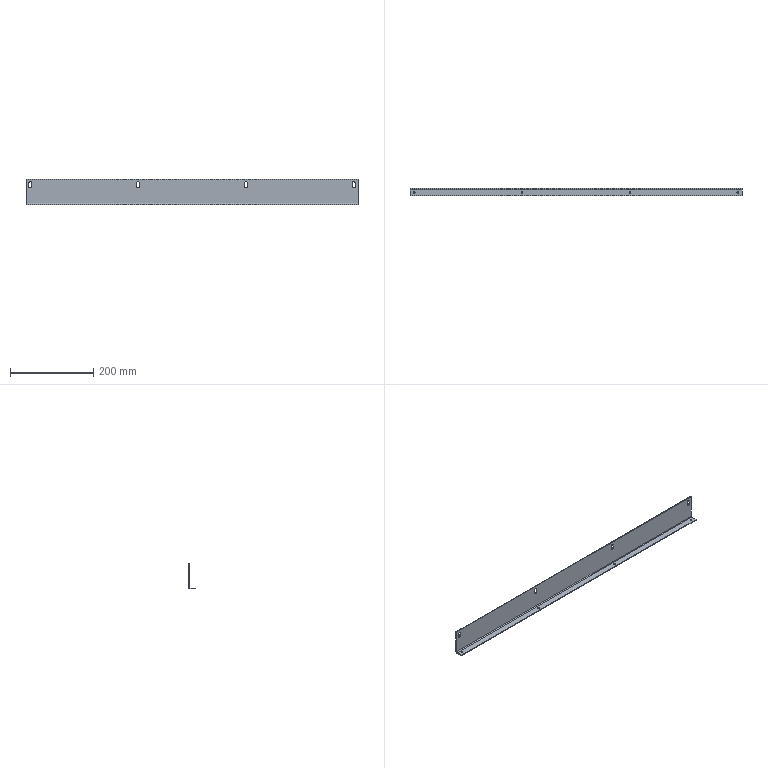Part | NX | features BREP 1 | 1 solid | 42 faces | box 800 x 18 x 62 mm | volume 121873 mm3 | cylinder 22 | plane 20 | commonest cylinder face diameters 7 x12 4.2 x8 4 x1 8 x1
STEP:
#1=CARTESIAN_POINT('',(393.5,0.,-9.5));
#2=VERTEX_POINT('',#1);
#3=CARTESIAN_POINT('',(393.5,-2.,-9.5));
#4=VERTEX_POINT('',#3);
#5=CARTESIAN_POINT('',(393.5,-18.,-9.5));
#6=DIRECTION('',(0.,-1.,0.));
#7=VECTOR('',#6,1000.);
#8=LINE('',#5,#7);
#9=EDGE_CURVE('',#2,#4,#8,.T.);
#10=ORIENTED_EDGE('',*,*,#9,.F.);
#11=CARTESIAN_POINT('',(393.5,0.,-17.5));
#12=VERTEX_POINT('',#11);
#13=CARTESIAN_POINT('',(393.5,0.,-9.5));
#14=DIRECTION('',(0.,0.,-1.));
#15=VECTOR('',#14,1000.);
#16=LINE('',#13,#15);
#17=EDGE_CURVE('',#2,#12,#16,.T.);
#18=ORIENTED_EDGE('',*,*,#17,.T.);
#19=CARTESIAN_POINT('',(393.5,-2.,-17.5));
#20=VERTEX_POINT('',#19);
#21=CARTESIAN_POINT('',(393.5,-18.,-17.5));
#22=DIRECTION('',(0.,-1.,0.));
#23=VECTOR('',#22,1000.);
#24=LINE('',#21,#23);
#25=EDGE_CURVE('',#12,#20,#24,.T.);
#26=ORIENTED_EDGE('',*,*,#25,.T.);
#27=CARTESIAN_POINT('',(393.5,-2.,0.));
#28=DIRECTION('',(0.,0.,-1.));
#29=VECTOR('',#28,1000.);
#30=LINE('',#27,#29);
#31=EDGE_CURVE('',#4,#20,#30,.T.);
#32=ORIENTED_EDGE('',*,*,#31,.F.);
#33=EDGE_LOOP('',(#10,#18,#26,#32));
#34=FACE_BOUND('',#33,.T.);
#35=CARTESIAN_POINT('',(393.5,-18.,-9.5));
#36=DIRECTION('',(1.,0.,0.));
#37=DIRECTION('',(0.,1.,0.));
#38=AXIS2_PLACEMENT_3D('',#35,#36,#37);
#39=PLANE('',#38);
#40=ADVANCED_FACE('',(#34),#39,.F.);
#41=CARTESIAN_POINT('',(386.5,-2.,-17.5));
#42=VERTEX_POINT('',#41);
#43=CARTESIAN_POINT('',(386.5,0.,-17.5));
#44=VERTEX_POINT('',#43);
#45=CARTESIAN_POINT('',(386.5,0.,-17.5));
#46=DIRECTION('',(0.,1.,0.));
#47=VECTOR('',#46,1000.);
#48=LINE('',#45,#47);
#49=EDGE_CURVE('',#42,#44,#48,.T.);
#50=ORIENTED_EDGE('',*,*,#49,.T.);
#51=CARTESIAN_POINT('',(386.5,0.,-9.5));
#52=VERTEX_POINT('',#51);
#53=CARTESIAN_POINT('',(386.5,0.,-9.5));
#54=DIRECTION('',(0.,0.,-1.));
#55=VECTOR('',#54,1000.);
#56=LINE('',#53,#55);
#57=EDGE_CURVE('',#52,#44,#56,.T.);
#58=ORIENTED_EDGE('',*,*,#57,.F.);
#59=CARTESIAN_POINT('',(386.5,-2.,-9.5));
#60=VERTEX_POINT('',#59);
#61=CARTESIAN_POINT('',(386.5,0.,-9.5));
#62=DIRECTION('',(0.,-1.,0.));
#63=VECTOR('',#62,1000.);
#64=LINE('',#61,#63);
#65=EDGE_CURVE('',#52,#60,#64,.T.);
#66=ORIENTED_EDGE('',*,*,#65,.T.);
#67=CARTESIAN_POINT('',(386.5,-2.,0.));
#68=DIRECTION('',(0.,0.,1.));
#69=VECTOR('',#68,1000.);
#70=LINE('',#67,#69);
#71=EDGE_CURVE('',#42,#60,#70,.T.);
#72=ORIENTED_EDGE('',*,*,#71,.F.);
#73=EDGE_LOOP('',(#50,#58,#66,#72));
#74=FACE_BOUND('',#73,.T.);
#75=CARTESIAN_POINT('',(386.5,0.,-9.5));
#76=DIRECTION('',(-1.,0.,0.));
#77=DIRECTION('',(0.,0.,1.));
#78=AXIS2_PLACEMENT_3D('',#75,#76,#77);
#79=PLANE('',#78);
#80=ADVANCED_FACE('',(#74),#79,.F.);
#81=CARTESIAN_POINT('',(390.,-2.,-6.));
#82=VERTEX_POINT('',#81);
#83=CARTESIAN_POINT('',(390.,0.,-6.));
#84=VERTEX_POINT('',#83);
#85=CARTESIAN_POINT('',(390.,0.,-6.));
#86=DIRECTION('',(0.,1.,0.));
#87=VECTOR('',#86,1000.);
#88=LINE('',#85,#87);
#89=EDGE_CURVE('',#82,#84,#88,.T.);
#90=ORIENTED_EDGE('',*,*,#89,.F.);
#91=CARTESIAN_POINT('',(390.,-2.,-9.5));
#92=DIRECTION('',(0.,1.,0.));
#93=DIRECTION('',(0.,0.,1.));
#94=AXIS2_PLACEMENT_3D('',#91,#92,#93);
#95=CIRCLE('',#94,3.5);
#96=EDGE_CURVE('',#60,#82,#95,.T.);
#97=ORIENTED_EDGE('',*,*,#96,.F.);
#98=ORIENTED_EDGE('',*,*,#65,.F.);
#99=CARTESIAN_POINT('',(390.,0.,-9.5));
#100=DIRECTION('',(0.,1.,0.));
#101=DIRECTION('',(0.,0.,1.));
#102=AXIS2_PLACEMENT_3D('',#99,#100,#101);
#103=CIRCLE('',#102,3.5);
#104=EDGE_CURVE('',#52,#84,#103,.T.);
#105=ORIENTED_EDGE('',*,*,#104,.T.);
#106=EDGE_LOOP('',(#90,#97,#98,#105));
#107=FACE_BOUND('',#106,.T.);
#108=CARTESIAN_POINT('',(390.,0.,-9.5));
#109=DIRECTION('',(0.,1.,0.));
#110=DIRECTION('',(0.,0.,1.));
#111=AXIS2_PLACEMENT_3D('',#108,#109,#110);
#112=CYLINDRICAL_SURFACE('',#111,3.5);
#113=ADVANCED_FACE('',(#107),#112,.F.);
#114=ORIENTED_EDGE('',*,*,#25,.F.);
#115=CARTESIAN_POINT('',(390.,0.,-17.5));
#116=DIRECTION('',(0.,1.,0.));
#117=DIRECTION('',(0.,0.,1.));
#118=AXIS2_PLACEMENT_3D('',#115,#116,#117);
#119=CIRCLE('',#118,3.5);
#120=EDGE_CURVE('',#12,#44,#119,.T.);
#121=ORIENTED_EDGE('',*,*,#120,.T.);
#122=ORIENTED_EDGE('',*,*,#49,.F.);
#123=CARTESIAN_POINT('',(390.,-2.,-17.5));
#124=DIRECTION('',(0.,1.,0.));
#125=DIRECTION('',(0.,0.,1.));
#126=AXIS2_PLACEMENT_3D('',#123,#124,#125);
#127=CIRCLE('',#126,3.5);
#128=EDGE_CURVE('',#20,#42,#127,.T.);
#129=ORIENTED_EDGE('',*,*,#128,.F.);
#130=EDGE_LOOP('',(#114,#121,#122,#129));
#131=FACE_BOUND('',#130,.T.);
#132=CARTESIAN_POINT('',(390.,0.,-17.5));
#133=DIRECTION('',(0.,1.,0.));
#134=DIRECTION('',(0.,0.,1.));
#135=AXIS2_PLACEMENT_3D('',#132,#133,#134);
#136=CYLINDRICAL_SURFACE('',#135,3.5);
#137=ADVANCED_FACE('',(#131),#136,.F.);
#138=CARTESIAN_POINT('',(133.5,0.,-9.5));
#139=VERTEX_POINT('',#138);
#140=CARTESIAN_POINT('',(133.5,-2.,-9.5));
#141=VERTEX_POINT('',#140);
#142=CARTESIAN_POINT('',(133.5,-18.,-9.5));
#143=DIRECTION('',(0.,-1.,0.));
#144=VECTOR('',#143,1000.);
#145=LINE('',#142,#144);
#146=EDGE_CURVE('',#139,#141,#145,.T.);
#147=ORIENTED_EDGE('',*,*,#146,.F.);
#148=CARTESIAN_POINT('',(133.5,0.,-17.5));
#149=VERTEX_POINT('',#148);
#150=CARTESIAN_POINT('',(133.5,0.,-9.5));
#151=DIRECTION('',(0.,0.,-1.));
#152=VECTOR('',#151,1000.);
#153=LINE('',#150,#152);
#154=EDGE_CURVE('',#139,#149,#153,.T.);
#155=ORIENTED_EDGE('',*,*,#154,.T.);
#156=CARTESIAN_POINT('',(133.5,-2.,-17.5));
#157=VERTEX_POINT('',#156);
#158=CARTESIAN_POINT('',(133.5,-18.,-17.5));
#159=DIRECTION('',(0.,-1.,0.));
#160=VECTOR('',#159,1000.);
#161=LINE('',#158,#160);
#162=EDGE_CURVE('',#149,#157,#161,.T.);
#163=ORIENTED_EDGE('',*,*,#162,.T.);
#164=CARTESIAN_POINT('',(133.5,-2.,0.));
#165=DIRECTION('',(0.,0.,-1.));
#166=VECTOR('',#165,1000.);
#167=LINE('',#164,#166);
#168=EDGE_CURVE('',#141,#157,#167,.T.);
#169=ORIENTED_EDGE('',*,*,#168,.F.);
#170=EDGE_LOOP('',(#147,#155,#163,#169));
#171=FACE_BOUND('',#170,.T.);
#172=CARTESIAN_POINT('',(133.5,-18.,-9.5));
#173=DIRECTION('',(1.,0.,0.));
#174=DIRECTION('',(0.,1.,0.));
#175=AXIS2_PLACEMENT_3D('',#172,#173,#174);
#176=PLANE('',#175);
#177=ADVANCED_FACE('',(#171),#176,.F.);
#178=CARTESIAN_POINT('',(126.5,-2.,-17.5));
#179=VERTEX_POINT('',#178);
#180=CARTESIAN_POINT('',(126.5,0.,-17.5));
#181=VERTEX_POINT('',#180);
#182=CARTESIAN_POINT('',(126.5,0.,-17.5));
#183=DIRECTION('',(0.,1.,0.));
#184=VECTOR('',#183,1000.);
#185=LINE('',#182,#184);
#186=EDGE_CURVE('',#179,#181,#185,.T.);
#187=ORIENTED_EDGE('',*,*,#186,.T.);
#188=CARTESIAN_POINT('',(126.5,0.,-9.5));
#189=VERTEX_POINT('',#188);
#190=CARTESIAN_POINT('',(126.5,0.,-9.5));
#191=DIRECTION('',(0.,0.,-1.));
#192=VECTOR('',#191,1000.);
#193=LINE('',#190,#192);
#194=EDGE_CURVE('',#189,#181,#193,.T.);
#195=ORIENTED_EDGE('',*,*,#194,.F.);
#196=CARTESIAN_POINT('',(126.5,-2.,-9.5));
#197=VERTEX_POINT('',#196);
#198=CARTESIAN_POINT('',(126.5,0.,-9.5));
#199=DIRECTION('',(0.,-1.,0.));
#200=VECTOR('',#199,1000.);
#201=LINE('',#198,#200);
#202=EDGE_CURVE('',#189,#197,#201,.T.);
#203=ORIENTED_EDGE('',*,*,#202,.T.);
#204=CARTESIAN_POINT('',(126.5,-2.,0.));
#205=DIRECTION('',(0.,0.,1.));
#206=VECTOR('',#205,1000.);
#207=LINE('',#204,#206);
#208=EDGE_CURVE('',#179,#197,#207,.T.);
#209=ORIENTED_EDGE('',*,*,#208,.F.);
#210=EDGE_LOOP('',(#187,#195,#203,#209));
#211=FACE_BOUND('',#210,.T.);
#212=CARTESIAN_POINT('',(126.5,0.,-9.5));
#213=DIRECTION('',(-1.,0.,0.));
#214=DIRECTION('',(0.,0.,1.));
#215=AXIS2_PLACEMENT_3D('',#212,#213,#214);
#216=PLANE('',#215);
#217=ADVANCED_FACE('',(#211),#216,.F.);
#218=CARTESIAN_POINT('',(130.,-2.,-6.));
#219=VERTEX_POINT('',#218);
#220=CARTESIAN_POINT('',(130.,0.,-6.));
#221=VERTEX_POINT('',#220);
#222=CARTESIAN_POINT('',(130.,0.,-6.));
#223=DIRECTION('',(0.,1.,0.));
#224=VECTOR('',#223,1000.);
#225=LINE('',#222,#224);
#226=EDGE_CURVE('',#219,#221,#225,.T.);
#227=ORIENTED_EDGE('',*,*,#226,.F.);
#228=CARTESIAN_POINT('',(130.,-2.,-9.5));
#229=DIRECTION('',(0.,1.,0.));
#230=DIRECTION('',(0.,0.,1.));
#231=AXIS2_PLACEMENT_3D('',#228,#229,#230);
#232=CIRCLE('',#231,3.5);
#233=EDGE_CURVE('',#197,#219,#232,.T.);
#234=ORIENTED_EDGE('',*,*,#233,.F.);
#235=ORIENTED_EDGE('',*,*,#202,.F.);
#236=CARTESIAN_POINT('',(130.,0.,-9.5));
#237=DIRECTION('',(0.,1.,0.));
#238=DIRECTION('',(0.,0.,1.));
#239=AXIS2_PLACEMENT_3D('',#236,#237,#238);
#240=CIRCLE('',#239,3.5);
#241=EDGE_CURVE('',#189,#221,#240,.T.);
#242=ORIENTED_EDGE('',*,*,#241,.T.);
#243=EDGE_LOOP('',(#227,#234,#235,#242));
#244=FACE_BOUND('',#243,.T.);
#245=CARTESIAN_POINT('',(130.,0.,-9.5));
#246=DIRECTION('',(0.,1.,0.));
#247=DIRECTION('',(0.,0.,1.));
#248=AXIS2_PLACEMENT_3D('',#245,#246,#247);
#249=CYLINDRICAL_SURFACE('',#248,3.5);
#250=ADVANCED_FACE('',(#244),#249,.F.);
#251=ORIENTED_EDGE('',*,*,#162,.F.);
#252=CARTESIAN_POINT('',(130.,0.,-17.5));
#253=DIRECTION('',(0.,1.,0.));
#254=DIRECTION('',(0.,0.,1.));
#255=AXIS2_PLACEMENT_3D('',#252,#253,#254);
#256=CIRCLE('',#255,3.5);
#257=EDGE_CURVE('',#149,#181,#256,.T.);
#258=ORIENTED_EDGE('',*,*,#257,.T.);
#259=ORIENTED_EDGE('',*,*,#186,.F.);
#260=CARTESIAN_POINT('',(130.,-2.,-17.5));
#261=DIRECTION('',(0.,1.,0.));
#262=DIRECTION('',(0.,0.,1.));
#263=AXIS2_PLACEMENT_3D('',#260,#261,#262);
#264=CIRCLE('',#263,3.5);
#265=EDGE_CURVE('',#157,#179,#264,.T.);
#266=ORIENTED_EDGE('',*,*,#265,.F.);
#267=EDGE_LOOP('',(#251,#258,#259,#266));
#268=FACE_BOUND('',#267,.T.);
#269=CARTESIAN_POINT('',(130.,0.,-17.5));
#270=DIRECTION('',(0.,1.,0.));
#271=DIRECTION('',(0.,0.,1.));
#272=AXIS2_PLACEMENT_3D('',#269,#270,#271);
#273=CYLINDRICAL_SURFACE('',#272,3.5);
#274=ADVANCED_FACE('',(#268),#273,.F.);
#275=CARTESIAN_POINT('',(-126.5,0.,-17.5));
#276=VERTEX_POINT('',#275);
#277=CARTESIAN_POINT('',(-126.5,-2.,-17.5));
#278=VERTEX_POINT('',#277);
#279=CARTESIAN_POINT('',(-126.5,-18.,-17.5));
#280=DIRECTION('',(0.,-1.,0.));
#281=VECTOR('',#280,1000.);
#282=LINE('',#279,#281);
#283=EDGE_CURVE('',#276,#278,#282,.T.);
#284=ORIENTED_EDGE('',*,*,#283,.F.);
#285=CARTESIAN_POINT('',(-133.5,0.,-17.5));
#286=VERTEX_POINT('',#285);
#287=CARTESIAN_POINT('',(-130.,0.,-17.5));
#288=DIRECTION('',(0.,1.,0.));
#289=DIRECTION('',(0.,0.,1.));
#290=AXIS2_PLACEMENT_3D('',#287,#288,#289);
#291=CIRCLE('',#290,3.5);
#292=EDGE_CURVE('',#276,#286,#291,.T.);
#293=ORIENTED_EDGE('',*,*,#292,.T.);
#294=CARTESIAN_POINT('',(-133.5,-2.,-17.5));
#295=VERTEX_POINT('',#294);
#296=CARTESIAN_POINT('',(-133.5,0.,-17.5));
#297=DIRECTION('',(0.,1.,0.));
#298=VECTOR('',#297,1000.);
#299=LINE('',#296,#298);
#300=EDGE_CURVE('',#295,#286,#299,.T.);
#301=ORIENTED_EDGE('',*,*,#300,.F.);
#302=CARTESIAN_POINT('',(-130.,-2.,-17.5));
#303=DIRECTION('',(0.,1.,0.));
#304=DIRECTION('',(0.,0.,1.));
#305=AXIS2_PLACEMENT_3D('',#302,#303,#304);
#306=CIRCLE('',#305,3.5);
#307=EDGE_CURVE('',#278,#295,#306,.T.);
#308=ORIENTED_EDGE('',*,*,#307,.F.);
#309=EDGE_LOOP('',(#284,#293,#301,#308));
#310=FACE_BOUND('',#309,.T.);
#311=CARTESIAN_POINT('',(-130.,0.,-17.5));
#312=DIRECTION('',(0.,1.,0.));
#313=DIRECTION('',(0.,0.,1.));
#314=AXIS2_PLACEMENT_3D('',#311,#312,#313);
#315=CYLINDRICAL_SURFACE('',#314,3.5);
#316=ADVANCED_FACE('',(#310),#315,.F.);
#317=CARTESIAN_POINT('',(-126.5,0.,-9.5));
#318=VERTEX_POINT('',#317);
#319=CARTESIAN_POINT('',(-126.5,-2.,-9.5));
#320=VERTEX_POINT('',#319);
#321=CARTESIAN_POINT('',(-126.5,-18.,-9.5));
#322=DIRECTION('',(0.,-1.,0.));
#323=VECTOR('',#322,1000.);
#324=LINE('',#321,#323);
#325=EDGE_CURVE('',#318,#320,#324,.T.);
#326=ORIENTED_EDGE('',*,*,#325,.F.);
#327=CARTESIAN_POINT('',(-126.5,0.,-9.5));
#328=DIRECTION('',(0.,0.,-1.));
#329=VECTOR('',#328,1000.);
#330=LINE('',#327,#329);
#331=EDGE_CURVE('',#318,#276,#330,.T.);
#332=ORIENTED_EDGE('',*,*,#331,.T.);
#333=ORIENTED_EDGE('',*,*,#283,.T.);
#334=CARTESIAN_POINT('',(-126.5,-2.,0.));
#335=DIRECTION('',(0.,0.,-1.));
#336=VECTOR('',#335,1000.);
#337=LINE('',#334,#336);
#338=EDGE_CURVE('',#320,#278,#337,.T.);
#339=ORIENTED_EDGE('',*,*,#338,.F.);
#340=EDGE_LOOP('',(#326,#332,#333,#339));
#341=FACE_BOUND('',#340,.T.);
#342=CARTESIAN_POINT('',(-126.5,-18.,-9.5));
#343=DIRECTION('',(1.,0.,0.));
#344=DIRECTION('',(0.,1.,0.));
#345=AXIS2_PLACEMENT_3D('',#342,#343,#344);
#346=PLANE('',#345);
#347=ADVANCED_FACE('',(#341),#346,.F.);
#348=ORIENTED_EDGE('',*,*,#300,.T.);
#349=CARTESIAN_POINT('',(-133.5,0.,-9.5));
#350=VERTEX_POINT('',#349);
#351=CARTESIAN_POINT('',(-133.5,0.,-9.5));
#352=DIRECTION('',(0.,0.,-1.));
#353=VECTOR('',#352,1000.);
#354=LINE('',#351,#353);
#355=EDGE_CURVE('',#350,#286,#354,.T.);
#356=ORIENTED_EDGE('',*,*,#355,.F.);
#357=CARTESIAN_POINT('',(-133.5,-2.,-9.5));
#358=VERTEX_POINT('',#357);
#359=CARTESIAN_POINT('',(-133.5,0.,-9.5));
#360=DIRECTION('',(0.,-1.,0.));
#361=VECTOR('',#360,1000.);
#362=LINE('',#359,#361);
#363=EDGE_CURVE('',#350,#358,#362,.T.);
#364=ORIENTED_EDGE('',*,*,#363,.T.);
#365=CARTESIAN_POINT('',(-133.5,-2.,0.));
#366=DIRECTION('',(0.,0.,1.));
#367=VECTOR('',#366,1000.);
#368=LINE('',#365,#367);
#369=EDGE_CURVE('',#295,#358,#368,.T.);
#370=ORIENTED_EDGE('',*,*,#369,.F.);
#371=EDGE_LOOP('',(#348,#356,#364,#370));
#372=FACE_BOUND('',#371,.T.);
#373=CARTESIAN_POINT('',(-133.5,0.,-9.5));
#374=DIRECTION('',(-1.,0.,0.));
#375=DIRECTION('',(0.,0.,1.));
#376=AXIS2_PLACEMENT_3D('',#373,#374,#375);
#377=PLANE('',#376);
#378=ADVANCED_FACE('',(#372),#377,.F.);
#379=CARTESIAN_POINT('',(-130.,-2.,-6.));
#380=VERTEX_POINT('',#379);
#381=CARTESIAN_POINT('',(-130.,0.,-6.));
#382=VERTEX_POINT('',#381);
#383=CARTESIAN_POINT('',(-130.,0.,-6.));
#384=DIRECTION('',(0.,1.,0.));
#385=VECTOR('',#384,1000.);
#386=LINE('',#383,#385);
#387=EDGE_CURVE('',#380,#382,#386,.T.);
#388=ORIENTED_EDGE('',*,*,#387,.F.);
#389=CARTESIAN_POINT('',(-130.,-2.,-9.5));
#390=DIRECTION('',(0.,1.,0.));
#391=DIRECTION('',(0.,0.,1.));
#392=AXIS2_PLACEMENT_3D('',#389,#390,#391);
#393=CIRCLE('',#392,3.5);
#394=EDGE_CURVE('',#358,#380,#393,.T.);
#395=ORIENTED_EDGE('',*,*,#394,.F.);
#396=ORIENTED_EDGE('',*,*,#363,.F.);
#397=CARTESIAN_POINT('',(-130.,0.,-9.5));
#398=DIRECTION('',(0.,1.,0.));
#399=DIRECTION('',(0.,0.,1.));
#400=AXIS2_PLACEMENT_3D('',#397,#398,#399);
#401=CIRCLE('',#400,3.5);
#402=EDGE_CURVE('',#350,#382,#401,.T.);
#403=ORIENTED_EDGE('',*,*,#402,.T.);
#404=EDGE_LOOP('',(#388,#395,#396,#403));
#405=FACE_BOUND('',#404,.T.);
#406=CARTESIAN_POINT('',(-130.,0.,-9.5));
#407=DIRECTION('',(0.,1.,0.));
#408=DIRECTION('',(0.,0.,1.));
#409=AXIS2_PLACEMENT_3D('',#406,#407,#408);
#410=CYLINDRICAL_SURFACE('',#409,3.5);
#411=ADVANCED_FACE('',(#405),#410,.F.);
#412=CARTESIAN_POINT('',(392.1,-10.5,-60.));
#413=VERTEX_POINT('',#412);
#414=CARTESIAN_POINT('',(392.1,-10.5,-62.));
#415=VERTEX_POINT('',#414);
#416=CARTESIAN_POINT('',(392.1,-10.5,-62.));
#417=DIRECTION('',(0.,0.,-1.));
#418=VECTOR('',#417,1000.);
#419=LINE('',#416,#418);
#420=EDGE_CURVE('',#413,#415,#419,.T.);
#421=ORIENTED_EDGE('',*,*,#420,.F.);
#422=CARTESIAN_POINT('',(387.9,-10.5,-60.));
#423=VERTEX_POINT('',#422);
#424=CARTESIAN_POINT('',(390.,-10.5,-60.));
#425=DIRECTION('',(0.,0.,-1.));
#426=DIRECTION('',(-1.,0.,0.));
#427=AXIS2_PLACEMENT_3D('',#424,#425,#426);
#428=CIRCLE('',#427,2.1);
#429=EDGE_CURVE('',#423,#413,#428,.T.);
#430=ORIENTED_EDGE('',*,*,#429,.F.);
#431=CARTESIAN_POINT('',(387.9,-10.5,-62.));
#432=VERTEX_POINT('',#431);
#433=CARTESIAN_POINT('',(387.9,-10.5,-62.));
#434=DIRECTION('',(0.,0.,-1.));
#435=VECTOR('',#434,1000.);
#436=LINE('',#433,#435);
#437=EDGE_CURVE('',#423,#432,#436,.T.);
#438=ORIENTED_EDGE('',*,*,#437,.T.);
#439=CARTESIAN_POINT('',(390.,-10.5,-62.));
#440=DIRECTION('',(0.,0.,-1.));
#441=DIRECTION('',(-1.,0.,0.));
#442=AXIS2_PLACEMENT_3D('',#439,#440,#441);
#443=CIRCLE('',#442,2.1);
#444=EDGE_CURVE('',#432,#415,#443,.T.);
#445=ORIENTED_EDGE('',*,*,#444,.T.);
#446=EDGE_LOOP('',(#421,#430,#438,#445));
#447=FACE_BOUND('',#446,.T.);
#448=CARTESIAN_POINT('',(390.,-10.5,-62.));
#449=DIRECTION('',(0.,0.,-1.));
#450=DIRECTION('',(-1.,0.,0.));
#451=AXIS2_PLACEMENT_3D('',#448,#449,#450);
#452=CYLINDRICAL_SURFACE('',#451,2.1);
#453=ADVANCED_FACE('',(#447),#452,.F.);
#454=CARTESIAN_POINT('',(132.1,-10.5,-60.));
#455=VERTEX_POINT('',#454);
#456=CARTESIAN_POINT('',(132.1,-10.5,-62.));
#457=VERTEX_POINT('',#456);
#458=CARTESIAN_POINT('',(132.1,-10.5,-62.));
#459=DIRECTION('',(0.,0.,-1.));
#460=VECTOR('',#459,1000.);
#461=LINE('',#458,#460);
#462=EDGE_CURVE('',#455,#457,#461,.T.);
#463=ORIENTED_EDGE('',*,*,#462,.F.);
#464=CARTESIAN_POINT('',(127.9,-10.5,-60.));
#465=VERTEX_POINT('',#464);
#466=CARTESIAN_POINT('',(130.,-10.5,-60.));
#467=DIRECTION('',(0.,0.,-1.));
#468=DIRECTION('',(-1.,0.,0.));
#469=AXIS2_PLACEMENT_3D('',#466,#467,#468);
#470=CIRCLE('',#469,2.1);
#471=EDGE_CURVE('',#465,#455,#470,.T.);
#472=ORIENTED_EDGE('',*,*,#471,.F.);
#473=CARTESIAN_POINT('',(127.9,-10.5,-62.));
#474=VERTEX_POINT('',#473);
#475=CARTESIAN_POINT('',(127.9,-10.5,-62.));
#476=DIRECTION('',(0.,0.,-1.));
#477=VECTOR('',#476,1000.);
#478=LINE('',#475,#477);
#479=EDGE_CURVE('',#465,#474,#478,.T.);
#480=ORIENTED_EDGE('',*,*,#479,.T.);
#481=CARTESIAN_POINT('',(130.,-10.5,-62.));
#482=DIRECTION('',(0.,0.,-1.));
#483=DIRECTION('',(-1.,0.,0.));
#484=AXIS2_PLACEMENT_3D('',#481,#482,#483);
#485=CIRCLE('',#484,2.1);
#486=EDGE_CURVE('',#474,#457,#485,.T.);
#487=ORIENTED_EDGE('',*,*,#486,.T.);
#488=EDGE_LOOP('',(#463,#472,#480,#487));
#489=FACE_BOUND('',#488,.T.);
#490=CARTESIAN_POINT('',(130.,-10.5,-62.));
#491=DIRECTION('',(0.,0.,-1.));
#492=DIRECTION('',(-1.,0.,0.));
#493=AXIS2_PLACEMENT_3D('',#490,#491,#492);
#494=CYLINDRICAL_SURFACE('',#493,2.1);
#495=ADVANCED_FACE('',(#489),#494,.F.);
#496=CARTESIAN_POINT('',(-127.9,-10.5,-60.));
#497=VERTEX_POINT('',#496);
#498=CARTESIAN_POINT('',(-127.9,-10.5,-62.));
#499=VERTEX_POINT('',#498);
#500=CARTESIAN_POINT('',(-127.9,-10.5,-62.));
#501=DIRECTION('',(0.,0.,-1.));
#502=VECTOR('',#501,1000.);
#503=LINE('',#500,#502);
#504=EDGE_CURVE('',#497,#499,#503,.T.);
#505=ORIENTED_EDGE('',*,*,#504,.F.);
#506=CARTESIAN_POINT('',(-132.1,-10.5,-60.));
#507=VERTEX_POINT('',#506);
#508=CARTESIAN_POINT('',(-130.,-10.5,-60.));
#509=DIRECTION('',(0.,0.,-1.));
#510=DIRECTION('',(-1.,0.,0.));
#511=AXIS2_PLACEMENT_3D('',#508,#509,#510);
#512=CIRCLE('',#511,2.1);
#513=EDGE_CURVE('',#507,#497,#512,.T.);
#514=ORIENTED_EDGE('',*,*,#513,.F.);
#515=CARTESIAN_POINT('',(-132.1,-10.5,-62.));
#516=VERTEX_POINT('',#515);
#517=CARTESIAN_POINT('',(-132.1,-10.5,-62.));
#518=DIRECTION('',(0.,0.,-1.));
#519=VECTOR('',#518,1000.);
#520=LINE('',#517,#519);
#521=EDGE_CURVE('',#507,#516,#520,.T.);
#522=ORIENTED_EDGE('',*,*,#521,.T.);
#523=CARTESIAN_POINT('',(-130.,-10.5,-62.));
#524=DIRECTION('',(0.,0.,-1.));
#525=DIRECTION('',(-1.,0.,0.));
#526=AXIS2_PLACEMENT_3D('',#523,#524,#525);
#527=CIRCLE('',#526,2.1);
#528=EDGE_CURVE('',#516,#499,#527,.T.);
#529=ORIENTED_EDGE('',*,*,#528,.T.);
#530=EDGE_LOOP('',(#505,#514,#522,#529));
#531=FACE_BOUND('',#530,.T.);
#532=CARTESIAN_POINT('',(-130.,-10.5,-62.));
#533=DIRECTION('',(0.,0.,-1.));
#534=DIRECTION('',(-1.,0.,0.));
#535=AXIS2_PLACEMENT_3D('',#532,#533,#534);
#536=CYLINDRICAL_SURFACE('',#535,2.1);
#537=ADVANCED_FACE('',(#531),#536,.F.);
#538=CARTESIAN_POINT('',(-393.5,-2.,-17.5));
#539=VERTEX_POINT('',#538);
#540=CARTESIAN_POINT('',(-393.5,0.,-17.5));
#541=VERTEX_POINT('',#540);
#542=CARTESIAN_POINT('',(-393.5,0.,-17.5));
#543=DIRECTION('',(0.,1.,0.));
#544=VECTOR('',#543,1000.);
#545=LINE('',#542,#544);
#546=EDGE_CURVE('',#539,#541,#545,.T.);
#547=ORIENTED_EDGE('',*,*,#546,.T.);
#548=CARTESIAN_POINT('',(-393.5,0.,-9.5));
#549=VERTEX_POINT('',#548);
#550=CARTESIAN_POINT('',(-393.5,0.,-9.5));
#551=DIRECTION('',(0.,0.,-1.));
#552=VECTOR('',#551,1000.);
#553=LINE('',#550,#552);
#554=EDGE_CURVE('',#549,#541,#553,.T.);
#555=ORIENTED_EDGE('',*,*,#554,.F.);
#556=CARTESIAN_POINT('',(-393.5,-2.,-9.5));
#557=VERTEX_POINT('',#556);
#558=CARTESIAN_POINT('',(-393.5,0.,-9.5));
#559=DIRECTION('',(0.,-1.,0.));
#560=VECTOR('',#559,1000.);
#561=LINE('',#558,#560);
#562=EDGE_CURVE('',#549,#557,#561,.T.);
#563=ORIENTED_EDGE('',*,*,#562,.T.);
#564=CARTESIAN_POINT('',(-393.5,-2.,0.));
#565=DIRECTION('',(0.,0.,1.));
#566=VECTOR('',#565,1000.);
#567=LINE('',#564,#566);
#568=EDGE_CURVE('',#539,#557,#567,.T.);
#569=ORIENTED_EDGE('',*,*,#568,.F.);
#570=EDGE_LOOP('',(#547,#555,#563,#569));
#571=FACE_BOUND('',#570,.T.);
#572=CARTESIAN_POINT('',(-393.5,0.,-9.5));
#573=DIRECTION('',(-1.,0.,0.));
#574=DIRECTION('',(0.,0.,1.));
#575=AXIS2_PLACEMENT_3D('',#572,#573,#574);
#576=PLANE('',#575);
#577=ADVANCED_FACE('',(#571),#576,.F.);
#578=CARTESIAN_POINT('',(-386.5,0.,-9.5));
#579=VERTEX_POINT('',#578);
#580=CARTESIAN_POINT('',(-386.5,-2.,-9.5));
#581=VERTEX_POINT('',#580);
#582=CARTESIAN_POINT('',(-386.5,-18.,-9.5));
#583=DIRECTION('',(0.,-1.,0.));
#584=VECTOR('',#583,1000.);
#585=LINE('',#582,#584);
#586=EDGE_CURVE('',#579,#581,#585,.T.);
#587=ORIENTED_EDGE('',*,*,#586,.F.);
#588=CARTESIAN_POINT('',(-386.5,0.,-17.5));
#589=VERTEX_POINT('',#588);
#590=CARTESIAN_POINT('',(-386.5,0.,-9.5));
#591=DIRECTION('',(0.,0.,-1.));
#592=VECTOR('',#591,1000.);
#593=LINE('',#590,#592);
#594=EDGE_CURVE('',#579,#589,#593,.T.);
#595=ORIENTED_EDGE('',*,*,#594,.T.);
#596=CARTESIAN_POINT('',(-386.5,-2.,-17.5));
#597=VERTEX_POINT('',#596);
#598=CARTESIAN_POINT('',(-386.5,-18.,-17.5));
#599=DIRECTION('',(0.,-1.,0.));
#600=VECTOR('',#599,1000.);
#601=LINE('',#598,#600);
#602=EDGE_CURVE('',#589,#597,#601,.T.);
#603=ORIENTED_EDGE('',*,*,#602,.T.);
#604=CARTESIAN_POINT('',(-386.5,-2.,0.));
#605=DIRECTION('',(0.,0.,-1.));
#606=VECTOR('',#605,1000.);
#607=LINE('',#604,#606);
#608=EDGE_CURVE('',#581,#597,#607,.T.);
#609=ORIENTED_EDGE('',*,*,#608,.F.);
#610=EDGE_LOOP('',(#587,#595,#603,#609));
#611=FACE_BOUND('',#610,.T.);
#612=CARTESIAN_POINT('',(-386.5,-18.,-9.5));
#613=DIRECTION('',(1.,0.,0.));
#614=DIRECTION('',(0.,1.,0.));
#615=AXIS2_PLACEMENT_3D('',#612,#613,#614);
#616=PLANE('',#615);
#617=ADVANCED_FACE('',(#611),#616,.F.);
#618=CARTESIAN_POINT('',(-390.,-2.,-6.));
#619=VERTEX_POINT('',#618);
#620=CARTESIAN_POINT('',(-390.,0.,-6.));
#621=VERTEX_POINT('',#620);
#622=CARTESIAN_POINT('',(-390.,0.,-6.));
#623=DIRECTION('',(0.,1.,0.));
#624=VECTOR('',#623,1000.);
#625=LINE('',#622,#624);
#626=EDGE_CURVE('',#619,#621,#625,.T.);
#627=ORIENTED_EDGE('',*,*,#626,.F.);
#628=CARTESIAN_POINT('',(-390.,-2.,-9.5));
#629=DIRECTION('',(0.,1.,0.));
#630=DIRECTION('',(0.,0.,1.));
#631=AXIS2_PLACEMENT_3D('',#628,#629,#630);
#632=CIRCLE('',#631,3.5);
#633=EDGE_CURVE('',#557,#619,#632,.T.);
#634=ORIENTED_EDGE('',*,*,#633,.F.);
#635=ORIENTED_EDGE('',*,*,#562,.F.);
#636=CARTESIAN_POINT('',(-390.,0.,-9.5));
#637=DIRECTION('',(0.,1.,0.));
#638=DIRECTION('',(0.,0.,1.));
#639=AXIS2_PLACEMENT_3D('',#636,#637,#638);
#640=CIRCLE('',#639,3.5);
#641=EDGE_CURVE('',#549,#621,#640,.T.);
#642=ORIENTED_EDGE('',*,*,#641,.T.);
#643=EDGE_LOOP('',(#627,#634,#635,#642));
#644=FACE_BOUND('',#643,.T.);
#645=CARTESIAN_POINT('',(-390.,0.,-9.5));
#646=DIRECTION('',(0.,1.,0.));
#647=DIRECTION('',(0.,0.,1.));
#648=AXIS2_PLACEMENT_3D('',#645,#646,#647);
#649=CYLINDRICAL_SURFACE('',#648,3.5);
#650=ADVANCED_FACE('',(#644),#649,.F.);
#651=ORIENTED_EDGE('',*,*,#602,.F.);
#652=CARTESIAN_POINT('',(-390.,0.,-17.5));
#653=DIRECTION('',(0.,1.,0.));
#654=DIRECTION('',(0.,0.,1.));
#655=AXIS2_PLACEMENT_3D('',#652,#653,#654);
#656=CIRCLE('',#655,3.5);
#657=EDGE_CURVE('',#589,#541,#656,.T.);
#658=ORIENTED_EDGE('',*,*,#657,.T.);
#659=ORIENTED_EDGE('',*,*,#546,.F.);
#660=CARTESIAN_POINT('',(-390.,-2.,-17.5));
#661=DIRECTION('',(0.,1.,0.));
#662=DIRECTION('',(0.,0.,1.));
#663=AXIS2_PLACEMENT_3D('',#660,#661,#662);
#664=CIRCLE('',#663,3.5);
#665=EDGE_CURVE('',#597,#539,#664,.T.);
#666=ORIENTED_EDGE('',*,*,#665,.F.);
#667=EDGE_LOOP('',(#651,#658,#659,#666));
#668=FACE_BOUND('',#667,.T.);
#669=CARTESIAN_POINT('',(-390.,0.,-17.5));
#670=DIRECTION('',(0.,1.,0.));
#671=DIRECTION('',(0.,0.,1.));
#672=AXIS2_PLACEMENT_3D('',#669,#670,#671);
#673=CYLINDRICAL_SURFACE('',#672,3.5);
#674=ADVANCED_FACE('',(#668),#673,.F.);
#675=CARTESIAN_POINT('',(-387.9,-10.5,-60.));
#676=VERTEX_POINT('',#675);
#677=CARTESIAN_POINT('',(-387.9,-10.5,-62.));
#678=VERTEX_POINT('',#677);
#679=CARTESIAN_POINT('',(-387.9,-10.5,-62.));
#680=DIRECTION('',(0.,0.,-1.));
#681=VECTOR('',#680,1000.);
#682=LINE('',#679,#681);
#683=EDGE_CURVE('',#676,#678,#682,.T.);
#684=ORIENTED_EDGE('',*,*,#683,.F.);
#685=CARTESIAN_POINT('',(-392.1,-10.5,-60.));
#686=VERTEX_POINT('',#685);
#687=CARTESIAN_POINT('',(-390.,-10.5,-60.));
#688=DIRECTION('',(0.,0.,-1.));
#689=DIRECTION('',(-1.,0.,0.));
#690=AXIS2_PLACEMENT_3D('',#687,#688,#689);
#691=CIRCLE('',#690,2.1);
#692=EDGE_CURVE('',#686,#676,#691,.T.);
#693=ORIENTED_EDGE('',*,*,#692,.F.);
#694=CARTESIAN_POINT('',(-392.1,-10.5,-62.));
#695=VERTEX_POINT('',#694);
#696=CARTESIAN_POINT('',(-392.1,-10.5,-62.));
#697=DIRECTION('',(0.,0.,-1.));
#698=VECTOR('',#697,1000.);
#699=LINE('',#696,#698);
#700=EDGE_CURVE('',#686,#695,#699,.T.);
#701=ORIENTED_EDGE('',*,*,#700,.T.);
#702=CARTESIAN_POINT('',(-390.,-10.5,-62.));
#703=DIRECTION('',(0.,0.,-1.));
#704=DIRECTION('',(-1.,0.,0.));
#705=AXIS2_PLACEMENT_3D('',#702,#703,#704);
#706=CIRCLE('',#705,2.1);
#707=EDGE_CURVE('',#695,#678,#706,.T.);
#708=ORIENTED_EDGE('',*,*,#707,.T.);
#709=EDGE_LOOP('',(#684,#693,#701,#708));
#710=FACE_BOUND('',#709,.T.);
#711=CARTESIAN_POINT('',(-390.,-10.5,-62.));
#712=DIRECTION('',(0.,0.,-1.));
#713=DIRECTION('',(-1.,0.,0.));
#714=AXIS2_PLACEMENT_3D('',#711,#712,#713);
#715=CYLINDRICAL_SURFACE('',#714,2.1);
#716=ADVANCED_FACE('',(#710),#715,.F.);
#717=CARTESIAN_POINT('',(-400.,-4.,-60.));
#718=VERTEX_POINT('',#717);
#719=CARTESIAN_POINT('',(-400.,-18.,-60.));
#720=VERTEX_POINT('',#719);
#721=CARTESIAN_POINT('',(-400.,0.,-60.));
#722=DIRECTION('',(0.,-1.,0.));
#723=VECTOR('',#722,1000.);
#724=LINE('',#721,#723);
#725=EDGE_CURVE('',#718,#720,#724,.T.);
#726=ORIENTED_EDGE('',*,*,#725,.F.);
#727=CARTESIAN_POINT('',(-400.,-4.,-62.));
#728=VERTEX_POINT('',#727);
#729=CARTESIAN_POINT('',(-400.,-4.,-60.));
#730=DIRECTION('',(0.,0.,-1.));
#731=VECTOR('',#730,1000.);
#732=LINE('',#729,#731);
#733=EDGE_CURVE('',#718,#728,#732,.T.);
#734=ORIENTED_EDGE('',*,*,#733,.T.);
#735=CARTESIAN_POINT('',(-400.,-18.,-62.));
#736=VERTEX_POINT('',#735);
#737=CARTESIAN_POINT('',(-400.,0.,-62.));
#738=DIRECTION('',(0.,-1.,0.));
#739=VECTOR('',#738,1000.);
#740=LINE('',#737,#739);
#741=EDGE_CURVE('',#728,#736,#740,.T.);
#742=ORIENTED_EDGE('',*,*,#741,.T.);
#743=CARTESIAN_POINT('',(-400.,-18.,-62.));
#744=DIRECTION('',(0.,0.,1.));
#745=VECTOR('',#744,1000.);
#746=LINE('',#743,#745);
#747=EDGE_CURVE('',#736,#720,#746,.T.);
#748=ORIENTED_EDGE('',*,*,#747,.T.);
#749=EDGE_LOOP('',(#726,#734,#742,#748));
#750=FACE_BOUND('',#749,.T.);
#751=CARTESIAN_POINT('',(-400.,-4.,-58.));
#752=DIRECTION('',(1.,0.,0.));
#753=DIRECTION('',(0.,0.,-1.));
#754=AXIS2_PLACEMENT_3D('',#751,#752,#753);
#755=PLANE('',#754);
#756=ADVANCED_FACE('',(#750),#755,.F.);
#757=CARTESIAN_POINT('',(400.,-2.,0.));
#758=VERTEX_POINT('',#757);
#759=CARTESIAN_POINT('',(400.,-2.,-58.));
#760=VERTEX_POINT('',#759);
#761=CARTESIAN_POINT('',(400.,-2.,0.));
#762=DIRECTION('',(0.,0.,-1.));
#763=VECTOR('',#762,1000.);
#764=LINE('',#761,#763);
#765=EDGE_CURVE('',#758,#760,#764,.T.);
#766=ORIENTED_EDGE('',*,*,#765,.T.);
#767=CARTESIAN_POINT('',(400.,0.,-58.));
#768=VERTEX_POINT('',#767);
#769=CARTESIAN_POINT('',(400.,-2.,-58.));
#770=DIRECTION('',(0.,1.,0.));
#771=VECTOR('',#770,1000.);
#772=LINE('',#769,#771);
#773=EDGE_CURVE('',#760,#768,#772,.T.);
#774=ORIENTED_EDGE('',*,*,#773,.T.);
#775=CARTESIAN_POINT('',(400.,0.,0.));
#776=VERTEX_POINT('',#775);
#777=CARTESIAN_POINT('',(400.,0.,0.));
#778=DIRECTION('',(0.,0.,-1.));
#779=VECTOR('',#778,1000.);
#780=LINE('',#777,#779);
#781=EDGE_CURVE('',#776,#768,#780,.T.);
#782=ORIENTED_EDGE('',*,*,#781,.F.);
#783=CARTESIAN_POINT('',(400.,-2.,0.));
#784=DIRECTION('',(0.,1.,0.));
#785=VECTOR('',#784,1000.);
#786=LINE('',#783,#785);
#787=EDGE_CURVE('',#758,#776,#786,.T.);
#788=ORIENTED_EDGE('',*,*,#787,.F.);
#789=EDGE_LOOP('',(#766,#774,#782,#788));
#790=FACE_BOUND('',#789,.T.);
#791=CARTESIAN_POINT('',(400.,-4.,-58.));
#792=DIRECTION('',(1.,0.,0.));
#793=DIRECTION('',(0.,0.,-1.));
#794=AXIS2_PLACEMENT_3D('',#791,#792,#793);
#795=PLANE('',#794);
#796=ADVANCED_FACE('',(#790),#795,.T.);
#797=CARTESIAN_POINT('',(-400.,-2.,-58.));
#798=VERTEX_POINT('',#797);
#799=CARTESIAN_POINT('',(-400.,-4.,-58.));
#800=DIRECTION('',(-1.,0.,0.));
#801=DIRECTION('',(0.,0.,-1.));
#802=AXIS2_PLACEMENT_3D('',#799,#800,#801);
#803=CIRCLE('',#802,2.);
#804=EDGE_CURVE('',#798,#718,#803,.T.);
#805=ORIENTED_EDGE('',*,*,#804,.T.);
#806=CARTESIAN_POINT('',(400.,-4.,-60.));
#807=VERTEX_POINT('',#806);
#808=CARTESIAN_POINT('',(400.,-4.,-60.));
#809=DIRECTION('',(-1.,0.,0.));
#810=VECTOR('',#809,1000.);
#811=LINE('',#808,#810);
#812=EDGE_CURVE('',#807,#718,#811,.T.);
#813=ORIENTED_EDGE('',*,*,#812,.F.);
#814=CARTESIAN_POINT('',(400.,-4.,-58.));
#815=DIRECTION('',(-1.,0.,0.));
#816=DIRECTION('',(0.,0.,-1.));
#817=AXIS2_PLACEMENT_3D('',#814,#815,#816);
#818=CIRCLE('',#817,2.);
#819=EDGE_CURVE('',#760,#807,#818,.T.);
#820=ORIENTED_EDGE('',*,*,#819,.F.);
#821=CARTESIAN_POINT('',(400.,-2.,-58.));
#822=DIRECTION('',(-1.,0.,0.));
#823=VECTOR('',#822,1000.);
#824=LINE('',#821,#823);
#825=EDGE_CURVE('',#760,#798,#824,.T.);
#826=ORIENTED_EDGE('',*,*,#825,.T.);
#827=EDGE_LOOP('',(#805,#813,#820,#826));
#828=FACE_BOUND('',#827,.T.);
#829=CARTESIAN_POINT('',(400.,-4.,-58.));
#830=DIRECTION('',(-1.,0.,0.));
#831=DIRECTION('',(0.,0.,1.));
#832=AXIS2_PLACEMENT_3D('',#829,#830,#831);
#833=CYLINDRICAL_SURFACE('',#832,2.);
#834=ADVANCED_FACE('',(#828),#833,.F.);
#835=CARTESIAN_POINT('',(-400.,-2.,0.));
#836=VERTEX_POINT('',#835);
#837=CARTESIAN_POINT('',(-400.,-2.,0.));
#838=DIRECTION('',(0.,0.,-1.));
#839=VECTOR('',#838,1000.);
#840=LINE('',#837,#839);
#841=EDGE_CURVE('',#836,#798,#840,.T.);
#842=ORIENTED_EDGE('',*,*,#841,.T.);
#843=ORIENTED_EDGE('',*,*,#825,.F.);
#844=ORIENTED_EDGE('',*,*,#765,.F.);
#845=CARTESIAN_POINT('',(400.,-2.,0.));
#846=DIRECTION('',(-1.,0.,0.));
#847=VECTOR('',#846,1000.);
#848=LINE('',#845,#847);
#849=EDGE_CURVE('',#758,#836,#848,.T.);
#850=ORIENTED_EDGE('',*,*,#849,.T.);
#851=EDGE_LOOP('',(#842,#843,#844,#850));
#852=FACE_BOUND('',#851,.T.);
#853=ORIENTED_EDGE('',*,*,#633,.T.);
#854=CARTESIAN_POINT('',(-390.,-2.,-9.5));
#855=DIRECTION('',(0.,1.,0.));
#856=DIRECTION('',(0.,0.,1.));
#857=AXIS2_PLACEMENT_3D('',#854,#855,#856);
#858=CIRCLE('',#857,3.5);
#859=EDGE_CURVE('',#619,#581,#858,.T.);
#860=ORIENTED_EDGE('',*,*,#859,.T.);
#861=ORIENTED_EDGE('',*,*,#608,.T.);
#862=ORIENTED_EDGE('',*,*,#665,.T.);
#863=ORIENTED_EDGE('',*,*,#568,.T.);
#864=EDGE_LOOP('',(#853,#860,#861,#862,#863));
#865=FACE_BOUND('',#864,.T.);
#866=ORIENTED_EDGE('',*,*,#369,.T.);
#867=ORIENTED_EDGE('',*,*,#394,.T.);
#868=CARTESIAN_POINT('',(-130.,-2.,-9.5));
#869=DIRECTION('',(0.,1.,0.));
#870=DIRECTION('',(0.,0.,1.));
#871=AXIS2_PLACEMENT_3D('',#868,#869,#870);
#872=CIRCLE('',#871,3.5);
#873=EDGE_CURVE('',#380,#320,#872,.T.);
#874=ORIENTED_EDGE('',*,*,#873,.T.);
#875=ORIENTED_EDGE('',*,*,#338,.T.);
#876=ORIENTED_EDGE('',*,*,#307,.T.);
#877=EDGE_LOOP('',(#866,#867,#874,#875,#876));
#878=FACE_BOUND('',#877,.T.);
#879=ORIENTED_EDGE('',*,*,#265,.T.);
#880=ORIENTED_EDGE('',*,*,#208,.T.);
#881=ORIENTED_EDGE('',*,*,#233,.T.);
#882=CARTESIAN_POINT('',(130.,-2.,-9.5));
#883=DIRECTION('',(0.,1.,0.));
#884=DIRECTION('',(0.,0.,1.));
#885=AXIS2_PLACEMENT_3D('',#882,#883,#884);
#886=CIRCLE('',#885,3.5);
#887=EDGE_CURVE('',#219,#141,#886,.T.);
#888=ORIENTED_EDGE('',*,*,#887,.T.);
#889=ORIENTED_EDGE('',*,*,#168,.T.);
#890=EDGE_LOOP('',(#879,#880,#881,#888,#889));
#891=FACE_BOUND('',#890,.T.);
#892=ORIENTED_EDGE('',*,*,#128,.T.);
#893=ORIENTED_EDGE('',*,*,#71,.T.);
#894=ORIENTED_EDGE('',*,*,#96,.T.);
#895=CARTESIAN_POINT('',(390.,-2.,-9.5));
#896=DIRECTION('',(0.,1.,0.));
#897=DIRECTION('',(0.,0.,1.));
#898=AXIS2_PLACEMENT_3D('',#895,#896,#897);
#899=CIRCLE('',#898,3.5);
#900=EDGE_CURVE('',#82,#4,#899,.T.);
#901=ORIENTED_EDGE('',*,*,#900,.T.);
#902=ORIENTED_EDGE('',*,*,#31,.T.);
#903=EDGE_LOOP('',(#892,#893,#894,#901,#902));
#904=FACE_BOUND('',#903,.T.);
#905=CARTESIAN_POINT('',(400.,-2.,0.));
#906=DIRECTION('',(0.,1.,0.));
#907=DIRECTION('',(0.,0.,1.));
#908=AXIS2_PLACEMENT_3D('',#905,#906,#907);
#909=PLANE('',#908);
#910=ADVANCED_FACE('',(#852,#865,#878,#891,#904),#909,.F.);
#911=CARTESIAN_POINT('',(-400.,0.,0.));
#912=VERTEX_POINT('',#911);
#913=CARTESIAN_POINT('',(-400.,-2.,0.));
#914=DIRECTION('',(0.,1.,0.));
#915=VECTOR('',#914,1000.);
#916=LINE('',#913,#915);
#917=EDGE_CURVE('',#836,#912,#916,.T.);
#918=ORIENTED_EDGE('',*,*,#917,.F.);
#919=ORIENTED_EDGE('',*,*,#849,.F.);
#920=ORIENTED_EDGE('',*,*,#787,.T.);
#921=CARTESIAN_POINT('',(400.,0.,0.));
#922=DIRECTION('',(-1.,0.,0.));
#923=VECTOR('',#922,1000.);
#924=LINE('',#921,#923);
#925=EDGE_CURVE('',#776,#912,#924,.T.);
#926=ORIENTED_EDGE('',*,*,#925,.T.);
#927=EDGE_LOOP('',(#918,#919,#920,#926));
#928=FACE_BOUND('',#927,.T.);
#929=CARTESIAN_POINT('',(400.,-2.,0.));
#930=DIRECTION('',(0.,0.,1.));
#931=DIRECTION('',(1.,0.,0.));
#932=AXIS2_PLACEMENT_3D('',#929,#930,#931);
#933=PLANE('',#932);
#934=ADVANCED_FACE('',(#928),#933,.T.);
#935=CARTESIAN_POINT('',(-400.,0.,-58.));
#936=VERTEX_POINT('',#935);
#937=CARTESIAN_POINT('',(-400.,-4.,-58.));
#938=DIRECTION('',(-1.,0.,0.));
#939=DIRECTION('',(0.,0.,-1.));
#940=AXIS2_PLACEMENT_3D('',#937,#938,#939);
#941=CIRCLE('',#940,4.);
#942=EDGE_CURVE('',#936,#728,#941,.T.);
#943=ORIENTED_EDGE('',*,*,#942,.F.);
#944=CARTESIAN_POINT('',(400.,0.,-58.));
#945=DIRECTION('',(-1.,0.,0.));
#946=VECTOR('',#945,1000.);
#947=LINE('',#944,#946);
#948=EDGE_CURVE('',#768,#936,#947,.T.);
#949=ORIENTED_EDGE('',*,*,#948,.F.);
#950=CARTESIAN_POINT('',(400.,-4.,-62.));
#951=VERTEX_POINT('',#950);
#952=CARTESIAN_POINT('',(400.,-4.,-58.));
#953=DIRECTION('',(-1.,0.,0.));
#954=DIRECTION('',(0.,0.,-1.));
#955=AXIS2_PLACEMENT_3D('',#952,#953,#954);
#956=CIRCLE('',#955,4.);
#957=EDGE_CURVE('',#768,#951,#956,.T.);
#958=ORIENTED_EDGE('',*,*,#957,.T.);
#959=CARTESIAN_POINT('',(400.,-4.,-62.));
#960=DIRECTION('',(-1.,0.,0.));
#961=VECTOR('',#960,1000.);
#962=LINE('',#959,#961);
#963=EDGE_CURVE('',#951,#728,#962,.T.);
#964=ORIENTED_EDGE('',*,*,#963,.T.);
#965=EDGE_LOOP('',(#943,#949,#958,#964));
#966=FACE_BOUND('',#965,.T.);
#967=CARTESIAN_POINT('',(400.,-4.,-58.));
#968=DIRECTION('',(-1.,0.,0.));
#969=DIRECTION('',(0.,0.,1.));
#970=AXIS2_PLACEMENT_3D('',#967,#968,#969);
#971=CYLINDRICAL_SURFACE('',#970,4.);
#972=ADVANCED_FACE('',(#966),#971,.T.);
#973=ORIENTED_EDGE('',*,*,#741,.F.);
#974=ORIENTED_EDGE('',*,*,#963,.F.);
#975=CARTESIAN_POINT('',(400.,-18.,-62.));
#976=VERTEX_POINT('',#975);
#977=CARTESIAN_POINT('',(400.,0.,-62.));
#978=DIRECTION('',(0.,-1.,0.));
#979=VECTOR('',#978,1000.);
#980=LINE('',#977,#979);
#981=EDGE_CURVE('',#951,#976,#980,.T.);
#982=ORIENTED_EDGE('',*,*,#981,.T.);
#983=CARTESIAN_POINT('',(400.,-18.,-62.));
#984=DIRECTION('',(-1.,0.,0.));
#985=VECTOR('',#984,1000.);
#986=LINE('',#983,#985);
#987=EDGE_CURVE('',#976,#736,#986,.T.);
#988=ORIENTED_EDGE('',*,*,#987,.T.);
#989=EDGE_LOOP('',(#973,#974,#982,#988));
#990=FACE_BOUND('',#989,.T.);
#991=ORIENTED_EDGE('',*,*,#707,.F.);
#992=CARTESIAN_POINT('',(-390.,-10.5,-62.));
#993=DIRECTION('',(0.,0.,-1.));
#994=DIRECTION('',(-1.,0.,0.));
#995=AXIS2_PLACEMENT_3D('',#992,#993,#994);
#996=CIRCLE('',#995,2.1);
#997=EDGE_CURVE('',#678,#695,#996,.T.);
#998=ORIENTED_EDGE('',*,*,#997,.F.);
#999=EDGE_LOOP('',(#991,#998));
#1000=FACE_BOUND('',#999,.T.);
#1001=ORIENTED_EDGE('',*,*,#528,.F.);
#1002=CARTESIAN_POINT('',(-130.,-10.5,-62.));
#1003=DIRECTION('',(0.,0.,-1.));
#1004=DIRECTION('',(-1.,0.,0.));
#1005=AXIS2_PLACEMENT_3D('',#1002,#1003,#1004);
#1006=CIRCLE('',#1005,2.1);
#1007=EDGE_CURVE('',#499,#516,#1006,.T.);
#1008=ORIENTED_EDGE('',*,*,#1007,.F.);
#1009=EDGE_LOOP('',(#1001,#1008));
#1010=FACE_BOUND('',#1009,.T.);
#1011=ORIENTED_EDGE('',*,*,#486,.F.);
#1012=CARTESIAN_POINT('',(130.,-10.5,-62.));
#1013=DIRECTION('',(0.,0.,-1.));
#1014=DIRECTION('',(-1.,0.,0.));
#1015=AXIS2_PLACEMENT_3D('',#1012,#1013,#1014);
#1016=CIRCLE('',#1015,2.1);
#1017=EDGE_CURVE('',#457,#474,#1016,.T.);
#1018=ORIENTED_EDGE('',*,*,#1017,.F.);
#1019=EDGE_LOOP('',(#1011,#1018));
#1020=FACE_BOUND('',#1019,.T.);
#1021=ORIENTED_EDGE('',*,*,#444,.F.);
#1022=CARTESIAN_POINT('',(390.,-10.5,-62.));
#1023=DIRECTION('',(0.,0.,-1.));
#1024=DIRECTION('',(-1.,0.,0.));
#1025=AXIS2_PLACEMENT_3D('',#1022,#1023,#1024);
#1026=CIRCLE('',#1025,2.1);
#1027=EDGE_CURVE('',#415,#432,#1026,.T.);
#1028=ORIENTED_EDGE('',*,*,#1027,.F.);
#1029=EDGE_LOOP('',(#1021,#1028));
#1030=FACE_BOUND('',#1029,.T.);
#1031=CARTESIAN_POINT('',(400.,0.,-62.));
#1032=DIRECTION('',(0.,0.,-1.));
#1033=DIRECTION('',(-1.,0.,0.));
#1034=AXIS2_PLACEMENT_3D('',#1031,#1032,#1033);
#1035=PLANE('',#1034);
#1036=ADVANCED_FACE('',(#990,#1000,#1010,#1020,#1030),#1035,.T.);
#1037=ORIENTED_EDGE('',*,*,#747,.F.);
#1038=ORIENTED_EDGE('',*,*,#987,.F.);
#1039=CARTESIAN_POINT('',(400.,-18.,-60.));
#1040=VERTEX_POINT('',#1039);
#1041=CARTESIAN_POINT('',(400.,-18.,-62.));
#1042=DIRECTION('',(0.,0.,1.));
#1043=VECTOR('',#1042,1000.);
#1044=LINE('',#1041,#1043);
#1045=EDGE_CURVE('',#976,#1040,#1044,.T.);
#1046=ORIENTED_EDGE('',*,*,#1045,.T.);
#1047=CARTESIAN_POINT('',(400.,-18.,-60.));
#1048=DIRECTION('',(-1.,0.,0.));
#1049=VECTOR('',#1048,1000.);
#1050=LINE('',#1047,#1049);
#1051=EDGE_CURVE('',#1040,#720,#1050,.T.);
#1052=ORIENTED_EDGE('',*,*,#1051,.T.);
#1053=EDGE_LOOP('',(#1037,#1038,#1046,#1052));
#1054=FACE_BOUND('',#1053,.T.);
#1055=CARTESIAN_POINT('',(400.,-18.,-62.));
#1056=DIRECTION('',(0.,-1.,0.));
#1057=DIRECTION('',(0.,0.,-1.));
#1058=AXIS2_PLACEMENT_3D('',#1055,#1056,#1057);
#1059=PLANE('',#1058);
#1060=ADVANCED_FACE('',(#1054),#1059,.T.);
#1061=ORIENTED_EDGE('',*,*,#725,.T.);
#1062=ORIENTED_EDGE('',*,*,#1051,.F.);
#1063=CARTESIAN_POINT('',(400.,0.,-60.));
#1064=DIRECTION('',(0.,-1.,0.));
#1065=VECTOR('',#1064,1000.);
#1066=LINE('',#1063,#1065);
#1067=EDGE_CURVE('',#807,#1040,#1066,.T.);
#1068=ORIENTED_EDGE('',*,*,#1067,.F.);
#1069=ORIENTED_EDGE('',*,*,#812,.T.);
#1070=EDGE_LOOP('',(#1061,#1062,#1068,#1069));
#1071=FACE_BOUND('',#1070,.T.);
#1072=ORIENTED_EDGE('',*,*,#692,.T.);
#1073=CARTESIAN_POINT('',(-390.,-10.5,-60.));
#1074=DIRECTION('',(0.,0.,-1.));
#1075=DIRECTION('',(-1.,0.,0.));
#1076=AXIS2_PLACEMENT_3D('',#1073,#1074,#1075);
#1077=CIRCLE('',#1076,2.1);
#1078=EDGE_CURVE('',#676,#686,#1077,.T.);
#1079=ORIENTED_EDGE('',*,*,#1078,.T.);
#1080=EDGE_LOOP('',(#1072,#1079));
#1081=FACE_BOUND('',#1080,.T.);
#1082=ORIENTED_EDGE('',*,*,#513,.T.);
#1083=CARTESIAN_POINT('',(-130.,-10.5,-60.));
#1084=DIRECTION('',(0.,0.,-1.));
#1085=DIRECTION('',(-1.,0.,0.));
#1086=AXIS2_PLACEMENT_3D('',#1083,#1084,#1085);
#1087=CIRCLE('',#1086,2.1);
#1088=EDGE_CURVE('',#497,#507,#1087,.T.);
#1089=ORIENTED_EDGE('',*,*,#1088,.T.);
#1090=EDGE_LOOP('',(#1082,#1089));
#1091=FACE_BOUND('',#1090,.T.);
#1092=ORIENTED_EDGE('',*,*,#471,.T.);
#1093=CARTESIAN_POINT('',(130.,-10.5,-60.));
#1094=DIRECTION('',(0.,0.,-1.));
#1095=DIRECTION('',(-1.,0.,0.));
#1096=AXIS2_PLACEMENT_3D('',#1093,#1094,#1095);
#1097=CIRCLE('',#1096,2.1);
#1098=EDGE_CURVE('',#455,#465,#1097,.T.);
#1099=ORIENTED_EDGE('',*,*,#1098,.T.);
#1100=EDGE_LOOP('',(#1092,#1099));
#1101=FACE_BOUND('',#1100,.T.);
#1102=ORIENTED_EDGE('',*,*,#429,.T.);
#1103=CARTESIAN_POINT('',(390.,-10.5,-60.));
#1104=DIRECTION('',(0.,0.,-1.));
#1105=DIRECTION('',(-1.,0.,0.));
#1106=AXIS2_PLACEMENT_3D('',#1103,#1104,#1105);
#1107=CIRCLE('',#1106,2.1);
#1108=EDGE_CURVE('',#413,#423,#1107,.T.);
#1109=ORIENTED_EDGE('',*,*,#1108,.T.);
#1110=EDGE_LOOP('',(#1102,#1109));
#1111=FACE_BOUND('',#1110,.T.);
#1112=CARTESIAN_POINT('',(400.,0.,-60.));
#1113=DIRECTION('',(0.,0.,-1.));
#1114=DIRECTION('',(-1.,0.,0.));
#1115=AXIS2_PLACEMENT_3D('',#1112,#1113,#1114);
#1116=PLANE('',#1115);
#1117=ADVANCED_FACE('',(#1071,#1081,#1091,#1101,#1111),#1116,.F.);
#1118=CARTESIAN_POINT('',(-400.,0.,0.));
#1119=DIRECTION('',(0.,0.,-1.));
#1120=VECTOR('',#1119,1000.);
#1121=LINE('',#1118,#1120);
#1122=EDGE_CURVE('',#912,#936,#1121,.T.);
#1123=ORIENTED_EDGE('',*,*,#1122,.T.);
#1124=CARTESIAN_POINT('',(-400.,0.,-58.));
#1125=DIRECTION('',(0.,-1.,0.));
#1126=VECTOR('',#1125,1000.);
#1127=LINE('',#1124,#1126);
#1128=EDGE_CURVE('',#936,#798,#1127,.T.);
#1129=ORIENTED_EDGE('',*,*,#1128,.T.);
#1130=ORIENTED_EDGE('',*,*,#841,.F.);
#1131=ORIENTED_EDGE('',*,*,#917,.T.);
#1132=EDGE_LOOP('',(#1123,#1129,#1130,#1131));
#1133=FACE_BOUND('',#1132,.T.);
#1134=CARTESIAN_POINT('',(-400.,-4.,-60.));
#1135=DIRECTION('',(-1.,0.,0.));
#1136=DIRECTION('',(0.,0.,1.));
#1137=AXIS2_PLACEMENT_3D('',#1134,#1135,#1136);
#1138=PLANE('',#1137);
#1139=ADVANCED_FACE('',(#1133),#1138,.T.);
#1140=ORIENTED_EDGE('',*,*,#1128,.F.);
#1141=ORIENTED_EDGE('',*,*,#942,.T.);
#1142=ORIENTED_EDGE('',*,*,#733,.F.);
#1143=ORIENTED_EDGE('',*,*,#804,.F.);
#1144=EDGE_LOOP('',(#1140,#1141,#1142,#1143));
#1145=FACE_BOUND('',#1144,.T.);
#1146=CARTESIAN_POINT('',(-400.,0.,-58.));
#1147=DIRECTION('',(-1.,0.,0.));
#1148=DIRECTION('',(0.,0.,1.));
#1149=AXIS2_PLACEMENT_3D('',#1146,#1147,#1148);
#1150=PLANE('',#1149);
#1151=ADVANCED_FACE('',(#1145),#1150,.T.);
#1152=ORIENTED_EDGE('',*,*,#981,.F.);
#1153=CARTESIAN_POINT('',(400.,-4.,-62.));
#1154=DIRECTION('',(0.,0.,1.));
#1155=VECTOR('',#1154,1000.);
#1156=LINE('',#1153,#1155);
#1157=EDGE_CURVE('',#951,#807,#1156,.T.);
#1158=ORIENTED_EDGE('',*,*,#1157,.T.);
#1159=ORIENTED_EDGE('',*,*,#1067,.T.);
#1160=ORIENTED_EDGE('',*,*,#1045,.F.);
#1161=EDGE_LOOP('',(#1152,#1158,#1159,#1160));
#1162=FACE_BOUND('',#1161,.T.);
#1163=CARTESIAN_POINT('',(400.,-2.,-58.));
#1164=DIRECTION('',(1.,0.,0.));
#1165=DIRECTION('',(0.,0.,-1.));
#1166=AXIS2_PLACEMENT_3D('',#1163,#1164,#1165);
#1167=PLANE('',#1166);
#1168=ADVANCED_FACE('',(#1162),#1167,.T.);
#1169=ORIENTED_EDGE('',*,*,#1157,.F.);
#1170=ORIENTED_EDGE('',*,*,#957,.F.);
#1171=ORIENTED_EDGE('',*,*,#773,.F.);
#1172=ORIENTED_EDGE('',*,*,#819,.T.);
#1173=EDGE_LOOP('',(#1169,#1170,#1171,#1172));
#1174=FACE_BOUND('',#1173,.T.);
#1175=CARTESIAN_POINT('',(400.,-4.,-62.));
#1176=DIRECTION('',(1.,0.,0.));
#1177=DIRECTION('',(0.,0.,-1.));
#1178=AXIS2_PLACEMENT_3D('',#1175,#1176,#1177);
#1179=PLANE('',#1178);
#1180=ADVANCED_FACE('',(#1174),#1179,.T.);
#1181=ORIENTED_EDGE('',*,*,#402,.F.);
#1182=ORIENTED_EDGE('',*,*,#355,.T.);
#1183=ORIENTED_EDGE('',*,*,#292,.F.);
#1184=ORIENTED_EDGE('',*,*,#331,.F.);
#1185=CARTESIAN_POINT('',(-130.,0.,-9.5));
#1186=DIRECTION('',(0.,1.,0.));
#1187=DIRECTION('',(0.,0.,1.));
#1188=AXIS2_PLACEMENT_3D('',#1185,#1186,#1187);
#1189=CIRCLE('',#1188,3.5);
#1190=EDGE_CURVE('',#382,#318,#1189,.T.);
#1191=ORIENTED_EDGE('',*,*,#1190,.F.);
#1192=EDGE_LOOP('',(#1181,#1182,#1183,#1184,#1191));
#1193=FACE_BOUND('',#1192,.T.);
#1194=ORIENTED_EDGE('',*,*,#641,.F.);
#1195=ORIENTED_EDGE('',*,*,#554,.T.);
#1196=ORIENTED_EDGE('',*,*,#657,.F.);
#1197=ORIENTED_EDGE('',*,*,#594,.F.);
#1198=CARTESIAN_POINT('',(-390.,0.,-9.5));
#1199=DIRECTION('',(0.,1.,0.));
#1200=DIRECTION('',(0.,0.,1.));
#1201=AXIS2_PLACEMENT_3D('',#1198,#1199,#1200);
#1202=CIRCLE('',#1201,3.5);
#1203=EDGE_CURVE('',#621,#579,#1202,.T.);
#1204=ORIENTED_EDGE('',*,*,#1203,.F.);
#1205=EDGE_LOOP('',(#1194,#1195,#1196,#1197,#1204));
#1206=FACE_BOUND('',#1205,.T.);
#1207=ORIENTED_EDGE('',*,*,#1122,.F.);
#1208=ORIENTED_EDGE('',*,*,#925,.F.);
#1209=ORIENTED_EDGE('',*,*,#781,.T.);
#1210=ORIENTED_EDGE('',*,*,#948,.T.);
#1211=EDGE_LOOP('',(#1207,#1208,#1209,#1210));
#1212=FACE_BOUND('',#1211,.T.);
#1213=ORIENTED_EDGE('',*,*,#154,.F.);
#1214=CARTESIAN_POINT('',(130.,0.,-9.5));
#1215=DIRECTION('',(0.,1.,0.));
#1216=DIRECTION('',(0.,0.,1.));
#1217=AXIS2_PLACEMENT_3D('',#1214,#1215,#1216);
#1218=CIRCLE('',#1217,3.5);
#1219=EDGE_CURVE('',#221,#139,#1218,.T.);
#1220=ORIENTED_EDGE('',*,*,#1219,.F.);
#1221=ORIENTED_EDGE('',*,*,#241,.F.);
#1222=ORIENTED_EDGE('',*,*,#194,.T.);
#1223=ORIENTED_EDGE('',*,*,#257,.F.);
#1224=EDGE_LOOP('',(#1213,#1220,#1221,#1222,#1223));
#1225=FACE_BOUND('',#1224,.T.);
#1226=ORIENTED_EDGE('',*,*,#17,.F.);
#1227=CARTESIAN_POINT('',(390.,0.,-9.5));
#1228=DIRECTION('',(0.,1.,0.));
#1229=DIRECTION('',(0.,0.,1.));
#1230=AXIS2_PLACEMENT_3D('',#1227,#1228,#1229);
#1231=CIRCLE('',#1230,3.5);
#1232=EDGE_CURVE('',#84,#2,#1231,.T.);
#1233=ORIENTED_EDGE('',*,*,#1232,.F.);
#1234=ORIENTED_EDGE('',*,*,#104,.F.);
#1235=ORIENTED_EDGE('',*,*,#57,.T.);
#1236=ORIENTED_EDGE('',*,*,#120,.F.);
#1237=EDGE_LOOP('',(#1226,#1233,#1234,#1235,#1236));
#1238=FACE_BOUND('',#1237,.T.);
#1239=CARTESIAN_POINT('',(400.,0.,0.));
#1240=DIRECTION('',(0.,1.,0.));
#1241=DIRECTION('',(0.,0.,1.));
#1242=AXIS2_PLACEMENT_3D('',#1239,#1240,#1241);
#1243=PLANE('',#1242);
#1244=ADVANCED_FACE('',(#1193,#1206,#1212,#1225,#1238),#1243,.T.);
#1245=ORIENTED_EDGE('',*,*,#1078,.F.);
#1246=ORIENTED_EDGE('',*,*,#683,.T.);
#1247=ORIENTED_EDGE('',*,*,#997,.T.);
#1248=ORIENTED_EDGE('',*,*,#700,.F.);
#1249=EDGE_LOOP('',(#1245,#1246,#1247,#1248));
#1250=FACE_BOUND('',#1249,.T.);
#1251=CARTESIAN_POINT('',(-390.,-10.5,-62.));
#1252=DIRECTION('',(0.,0.,-1.));
#1253=DIRECTION('',(-1.,0.,0.));
#1254=AXIS2_PLACEMENT_3D('',#1251,#1252,#1253);
#1255=CYLINDRICAL_SURFACE('',#1254,2.1);
#1256=ADVANCED_FACE('',(#1250),#1255,.F.);
#1257=ORIENTED_EDGE('',*,*,#859,.F.);
#1258=ORIENTED_EDGE('',*,*,#626,.T.);
#1259=ORIENTED_EDGE('',*,*,#1203,.T.);
#1260=ORIENTED_EDGE('',*,*,#586,.T.);
#1261=EDGE_LOOP('',(#1257,#1258,#1259,#1260));
#1262=FACE_BOUND('',#1261,.T.);
#1263=CARTESIAN_POINT('',(-390.,0.,-9.5));
#1264=DIRECTION('',(0.,1.,0.));
#1265=DIRECTION('',(0.,0.,1.));
#1266=AXIS2_PLACEMENT_3D('',#1263,#1264,#1265);
#1267=CYLINDRICAL_SURFACE('',#1266,3.5);
#1268=ADVANCED_FACE('',(#1262),#1267,.F.);
#1269=ORIENTED_EDGE('',*,*,#1088,.F.);
#1270=ORIENTED_EDGE('',*,*,#504,.T.);
#1271=ORIENTED_EDGE('',*,*,#1007,.T.);
#1272=ORIENTED_EDGE('',*,*,#521,.F.);
#1273=EDGE_LOOP('',(#1269,#1270,#1271,#1272));
#1274=FACE_BOUND('',#1273,.T.);
#1275=CARTESIAN_POINT('',(-130.,-10.5,-62.));
#1276=DIRECTION('',(0.,0.,-1.));
#1277=DIRECTION('',(-1.,0.,0.));
#1278=AXIS2_PLACEMENT_3D('',#1275,#1276,#1277);
#1279=CYLINDRICAL_SURFACE('',#1278,2.1);
#1280=ADVANCED_FACE('',(#1274),#1279,.F.);
#1281=ORIENTED_EDGE('',*,*,#1098,.F.);
#1282=ORIENTED_EDGE('',*,*,#462,.T.);
#1283=ORIENTED_EDGE('',*,*,#1017,.T.);
#1284=ORIENTED_EDGE('',*,*,#479,.F.);
#1285=EDGE_LOOP('',(#1281,#1282,#1283,#1284));
#1286=FACE_BOUND('',#1285,.T.);
#1287=CARTESIAN_POINT('',(130.,-10.5,-62.));
#1288=DIRECTION('',(0.,0.,-1.));
#1289=DIRECTION('',(-1.,0.,0.));
#1290=AXIS2_PLACEMENT_3D('',#1287,#1288,#1289);
#1291=CYLINDRICAL_SURFACE('',#1290,2.1);
#1292=ADVANCED_FACE('',(#1286),#1291,.F.);
#1293=ORIENTED_EDGE('',*,*,#1108,.F.);
#1294=ORIENTED_EDGE('',*,*,#420,.T.);
#1295=ORIENTED_EDGE('',*,*,#1027,.T.);
#1296=ORIENTED_EDGE('',*,*,#437,.F.);
#1297=EDGE_LOOP('',(#1293,#1294,#1295,#1296));
#1298=FACE_BOUND('',#1297,.T.);
#1299=CARTESIAN_POINT('',(390.,-10.5,-62.));
#1300=DIRECTION('',(0.,0.,-1.));
#1301=DIRECTION('',(-1.,0.,0.));
#1302=AXIS2_PLACEMENT_3D('',#1299,#1300,#1301);
#1303=CYLINDRICAL_SURFACE('',#1302,2.1);
#1304=ADVANCED_FACE('',(#1298),#1303,.F.);
#1305=ORIENTED_EDGE('',*,*,#873,.F.);
#1306=ORIENTED_EDGE('',*,*,#387,.T.);
#1307=ORIENTED_EDGE('',*,*,#1190,.T.);
#1308=ORIENTED_EDGE('',*,*,#325,.T.);
#1309=EDGE_LOOP('',(#1305,#1306,#1307,#1308));
#1310=FACE_BOUND('',#1309,.T.);
#1311=CARTESIAN_POINT('',(-130.,0.,-9.5));
#1312=DIRECTION('',(0.,1.,0.));
#1313=DIRECTION('',(0.,0.,1.));
#1314=AXIS2_PLACEMENT_3D('',#1311,#1312,#1313);
#1315=CYLINDRICAL_SURFACE('',#1314,3.5);
#1316=ADVANCED_FACE('',(#1310),#1315,.F.);
#1317=ORIENTED_EDGE('',*,*,#887,.F.);
#1318=ORIENTED_EDGE('',*,*,#226,.T.);
#1319=ORIENTED_EDGE('',*,*,#1219,.T.);
#1320=ORIENTED_EDGE('',*,*,#146,.T.);
#1321=EDGE_LOOP('',(#1317,#1318,#1319,#1320));
#1322=FACE_BOUND('',#1321,.T.);
#1323=CARTESIAN_POINT('',(130.,0.,-9.5));
#1324=DIRECTION('',(0.,1.,0.));
#1325=DIRECTION('',(0.,0.,1.));
#1326=AXIS2_PLACEMENT_3D('',#1323,#1324,#1325);
#1327=CYLINDRICAL_SURFACE('',#1326,3.5);
#1328=ADVANCED_FACE('',(#1322),#1327,.F.);
#1329=ORIENTED_EDGE('',*,*,#900,.F.);
#1330=ORIENTED_EDGE('',*,*,#89,.T.);
#1331=ORIENTED_EDGE('',*,*,#1232,.T.);
#1332=ORIENTED_EDGE('',*,*,#9,.T.);
#1333=EDGE_LOOP('',(#1329,#1330,#1331,#1332));
#1334=FACE_BOUND('',#1333,.T.);
#1335=CARTESIAN_POINT('',(390.,0.,-9.5));
#1336=DIRECTION('',(0.,1.,0.));
#1337=DIRECTION('',(0.,0.,1.));
#1338=AXIS2_PLACEMENT_3D('',#1335,#1336,#1337);
#1339=CYLINDRICAL_SURFACE('',#1338,3.5);
#1340=ADVANCED_FACE('',(#1334),#1339,.F.);
#1341=CLOSED_SHELL('',(#40,#80,#113,#137,#177,#217,#250,#274,#316,#347,#378,#411,#453,#495,#537,#577,#617,#650,#674,#716,#756,#796,#834,#910,#934,#972,#1036,#1060,#1117,#1139,#1151,#1168,#1180,#1244,#1256,#1268,#1280,#1292,#1304,#1316,#1328,#1340));
#1342=MANIFOLD_SOLID_BREP('',#1341);
#1343=(LENGTH_UNIT()NAMED_UNIT(*)SI_UNIT(.MILLI.,.METRE.));
#1344=UNCERTAINTY_MEASURE_WITH_UNIT(LENGTH_MEASURE(0.00001),#1343,'','');
#1345=(NAMED_UNIT(*)PLANE_ANGLE_UNIT()SI_UNIT($,.RADIAN.));
#1346=(NAMED_UNIT(*)SI_UNIT($,.STERADIAN.)SOLID_ANGLE_UNIT());
#1347=(GEOMETRIC_REPRESENTATION_CONTEXT(3)GLOBAL_UNCERTAINTY_ASSIGNED_CONTEXT((#1344))GLOBAL_UNIT_ASSIGNED_CONTEXT((#1343,#1345,#1346))REPRESENTATION_CONTEXT('',''));
#1348=ADVANCED_BREP_SHAPE_REPRESENTATION('',(#1342),#1347);